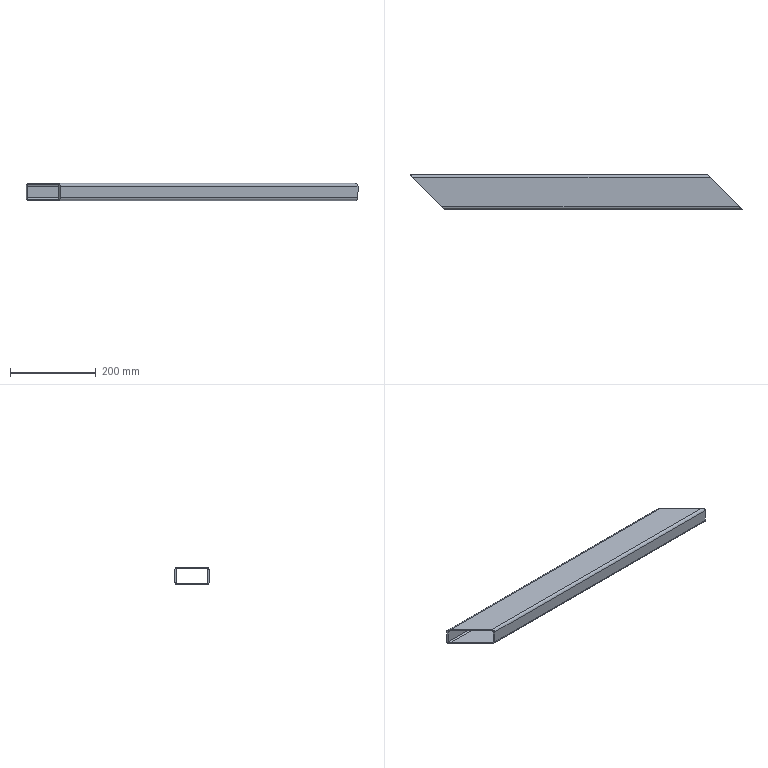Part | SolidWorks | features 3DProfileFeature 1, ICE 1, WeldMemberFeat 1, WeldmentFeature 1 | 1 solid | 18 faces | box 775 x 80 x 40 mm | volume 459272 mm3 | plane 10 | cylinder 8 | commonest cylinder face diameters 6 x4 12 x4
STEP:
#1=CARTESIAN_POINT('',(695.,40.,14.));
#2=VERTEX_POINT('',#1);
#3=CARTESIAN_POINT('',(0.,40.,14.));
#4=VERTEX_POINT('',#3);
#5=CARTESIAN_POINT('',(775.,40.,14.));
#6=DIRECTION('',(-1.,0.,0.));
#7=VECTOR('',#6,1000.);
#8=LINE('',#5,#7);
#9=EDGE_CURVE('',#2,#4,#8,.T.);
#10=ORIENTED_EDGE('',*,*,#9,.F.);
#11=CARTESIAN_POINT('',(695.,40.,-14.));
#12=VERTEX_POINT('',#11);
#13=CARTESIAN_POINT('',(695.,40.,-20.));
#14=DIRECTION('',(0.,0.,1.));
#15=VECTOR('',#14,1000.);
#16=LINE('',#13,#15);
#17=EDGE_CURVE('',#12,#2,#16,.T.);
#18=ORIENTED_EDGE('',*,*,#17,.F.);
#19=CARTESIAN_POINT('',(0.,40.,-14.));
#20=VERTEX_POINT('',#19);
#21=CARTESIAN_POINT('',(775.,40.,-14.));
#22=DIRECTION('',(-1.,0.,0.));
#23=VECTOR('',#22,1000.);
#24=LINE('',#21,#23);
#25=EDGE_CURVE('',#12,#20,#24,.T.);
#26=ORIENTED_EDGE('',*,*,#25,.T.);
#27=CARTESIAN_POINT('',(0.,40.,-14.));
#28=DIRECTION('',(0.,0.,1.));
#29=VECTOR('',#28,1000.);
#30=LINE('',#27,#29);
#31=EDGE_CURVE('',#20,#4,#30,.T.);
#32=ORIENTED_EDGE('',*,*,#31,.T.);
#33=EDGE_LOOP('',(#10,#18,#26,#32));
#34=FACE_OUTER_BOUND('',#33,.T.);
#35=CARTESIAN_POINT('',(775.,40.,-14.));
#36=DIRECTION('',(0.,-1.,0.));
#37=DIRECTION('',(0.,0.,-1.));
#38=AXIS2_PLACEMENT_3D('',#35,#36,#37);
#39=PLANE('',#38);
#40=ADVANCED_FACE('',(#34),#39,.F.);
#41=CARTESIAN_POINT('',(80.,-40.,-14.));
#42=VERTEX_POINT('',#41);
#43=CARTESIAN_POINT('',(80.,-40.,14.));
#44=VERTEX_POINT('',#43);
#45=CARTESIAN_POINT('',(80.,-40.,-20.));
#46=DIRECTION('',(0.,0.,1.));
#47=VECTOR('',#46,1000.);
#48=LINE('',#45,#47);
#49=EDGE_CURVE('',#42,#44,#48,.T.);
#50=ORIENTED_EDGE('',*,*,#49,.F.);
#51=CARTESIAN_POINT('',(775.,-40.,-14.));
#52=VERTEX_POINT('',#51);
#53=CARTESIAN_POINT('',(775.,-40.,-14.));
#54=DIRECTION('',(-1.,0.,0.));
#55=VECTOR('',#54,1000.);
#56=LINE('',#53,#55);
#57=EDGE_CURVE('',#52,#42,#56,.T.);
#58=ORIENTED_EDGE('',*,*,#57,.F.);
#59=CARTESIAN_POINT('',(775.,-40.,14.));
#60=VERTEX_POINT('',#59);
#61=CARTESIAN_POINT('',(775.,-40.,14.));
#62=DIRECTION('',(0.,0.,-1.));
#63=VECTOR('',#62,1000.);
#64=LINE('',#61,#63);
#65=EDGE_CURVE('',#60,#52,#64,.T.);
#66=ORIENTED_EDGE('',*,*,#65,.F.);
#67=CARTESIAN_POINT('',(775.,-40.,14.));
#68=DIRECTION('',(-1.,0.,0.));
#69=VECTOR('',#68,1000.);
#70=LINE('',#67,#69);
#71=EDGE_CURVE('',#60,#44,#70,.T.);
#72=ORIENTED_EDGE('',*,*,#71,.T.);
#73=EDGE_LOOP('',(#50,#58,#66,#72));
#74=FACE_OUTER_BOUND('',#73,.T.);
#75=CARTESIAN_POINT('',(775.,-40.,14.));
#76=DIRECTION('',(0.,1.,0.));
#77=DIRECTION('',(0.,0.,1.));
#78=AXIS2_PLACEMENT_3D('',#75,#76,#77);
#79=PLANE('',#78);
#80=ADVANCED_FACE('',(#74),#79,.F.);
#81=CARTESIAN_POINT('',(701.,34.,-20.));
#82=VERTEX_POINT('',#81);
#83=CARTESIAN_POINT('',(6.,34.,-20.));
#84=VERTEX_POINT('',#83);
#85=CARTESIAN_POINT('',(775.,34.,-20.));
#86=DIRECTION('',(-1.,0.,0.));
#87=VECTOR('',#86,1000.);
#88=LINE('',#85,#87);
#89=EDGE_CURVE('',#82,#84,#88,.T.);
#90=ORIENTED_EDGE('',*,*,#89,.F.);
#91=CARTESIAN_POINT('',(769.,-34.,-20.));
#92=VERTEX_POINT('',#91);
#93=CARTESIAN_POINT('',(367.5,367.5,-20.));
#94=DIRECTION('',(0.7071,-0.7071,0.));
#95=VECTOR('',#94,1000.);
#96=LINE('',#93,#95);
#97=EDGE_CURVE('',#82,#92,#96,.T.);
#98=ORIENTED_EDGE('',*,*,#97,.T.);
#99=CARTESIAN_POINT('',(74.,-34.,-20.));
#100=VERTEX_POINT('',#99);
#101=CARTESIAN_POINT('',(775.,-34.,-20.));
#102=DIRECTION('',(-1.,0.,0.));
#103=VECTOR('',#102,1000.);
#104=LINE('',#101,#103);
#105=EDGE_CURVE('',#92,#100,#104,.T.);
#106=ORIENTED_EDGE('',*,*,#105,.T.);
#107=CARTESIAN_POINT('',(20.,20.,-20.));
#108=DIRECTION('',(0.7071,-0.7071,0.));
#109=VECTOR('',#108,1000.);
#110=LINE('',#107,#109);
#111=EDGE_CURVE('',#84,#100,#110,.T.);
#112=ORIENTED_EDGE('',*,*,#111,.F.);
#113=EDGE_LOOP('',(#90,#98,#106,#112));
#114=FACE_OUTER_BOUND('',#113,.T.);
#115=CARTESIAN_POINT('',(775.,34.,-20.));
#116=DIRECTION('',(0.,0.,1.));
#117=DIRECTION('',(1.,0.,0.));
#118=AXIS2_PLACEMENT_3D('',#115,#116,#117);
#119=PLANE('',#118);
#120=ADVANCED_FACE('',(#114),#119,.F.);
#121=ORIENTED_EDGE('',*,*,#105,.F.);
#122=CARTESIAN_POINT('',(769.,-34.,-20.));
#123=CARTESIAN_POINT('',(772.515,-37.515,-20.));
#124=CARTESIAN_POINT('',(775.,-40.,-17.515));
#125=CARTESIAN_POINT('',(775.,-40.,-14.));
#126=(BOUNDED_CURVE()B_SPLINE_CURVE(3,(#122,#123,#124,#125),.UNSPECIFIED.,.F.,.F.)B_SPLINE_CURVE_WITH_KNOTS((4,4),(1.571,3.142),.UNSPECIFIED.)CURVE()GEOMETRIC_REPRESENTATION_ITEM()RATIONAL_B_SPLINE_CURVE((1.,0.8047,0.8047,1.))REPRESENTATION_ITEM(''));
#127=EDGE_CURVE('',#92,#52,#126,.T.);
#128=ORIENTED_EDGE('',*,*,#127,.T.);
#129=ORIENTED_EDGE('',*,*,#57,.T.);
#130=CARTESIAN_POINT('',(74.,-34.,-20.));
#131=CARTESIAN_POINT('',(77.515,-37.515,-20.));
#132=CARTESIAN_POINT('',(80.,-40.,-17.515));
#133=CARTESIAN_POINT('',(80.,-40.,-14.));
#134=(BOUNDED_CURVE()B_SPLINE_CURVE(3,(#130,#131,#132,#133),.UNSPECIFIED.,.F.,.F.)B_SPLINE_CURVE_WITH_KNOTS((4,4),(1.571,3.142),.UNSPECIFIED.)CURVE()GEOMETRIC_REPRESENTATION_ITEM()RATIONAL_B_SPLINE_CURVE((1.,0.8047,0.8047,1.))REPRESENTATION_ITEM(''));
#135=EDGE_CURVE('',#100,#42,#134,.T.);
#136=ORIENTED_EDGE('',*,*,#135,.F.);
#137=EDGE_LOOP('',(#121,#128,#129,#136));
#138=FACE_OUTER_BOUND('',#137,.T.);
#139=CARTESIAN_POINT('',(775.,-34.,-14.));
#140=DIRECTION('',(-1.,0.,0.));
#141=DIRECTION('',(0.,0.,1.));
#142=AXIS2_PLACEMENT_3D('',#139,#140,#141);
#143=CYLINDRICAL_SURFACE('',#142,6.);
#144=ADVANCED_FACE('',(#138),#143,.T.);
#145=ORIENTED_EDGE('',*,*,#71,.F.);
#146=CARTESIAN_POINT('',(769.,-34.,20.));
#147=VERTEX_POINT('',#146);
#148=CARTESIAN_POINT('',(775.,-40.,14.));
#149=CARTESIAN_POINT('',(775.,-40.,17.515));
#150=CARTESIAN_POINT('',(772.515,-37.515,20.));
#151=CARTESIAN_POINT('',(769.,-34.,20.));
#152=(BOUNDED_CURVE()B_SPLINE_CURVE(3,(#148,#149,#150,#151),.UNSPECIFIED.,.F.,.F.)B_SPLINE_CURVE_WITH_KNOTS((4,4),(3.142,4.712),.UNSPECIFIED.)CURVE()GEOMETRIC_REPRESENTATION_ITEM()RATIONAL_B_SPLINE_CURVE((1.,0.8047,0.8047,1.))REPRESENTATION_ITEM(''));
#153=EDGE_CURVE('',#60,#147,#152,.T.);
#154=ORIENTED_EDGE('',*,*,#153,.T.);
#155=CARTESIAN_POINT('',(74.,-34.,20.));
#156=VERTEX_POINT('',#155);
#157=CARTESIAN_POINT('',(775.,-34.,20.));
#158=DIRECTION('',(-1.,0.,0.));
#159=VECTOR('',#158,1000.);
#160=LINE('',#157,#159);
#161=EDGE_CURVE('',#147,#156,#160,.T.);
#162=ORIENTED_EDGE('',*,*,#161,.T.);
#163=CARTESIAN_POINT('',(80.,-40.,14.));
#164=CARTESIAN_POINT('',(80.,-40.,17.515));
#165=CARTESIAN_POINT('',(77.515,-37.515,20.));
#166=CARTESIAN_POINT('',(74.,-34.,20.));
#167=(BOUNDED_CURVE()B_SPLINE_CURVE(3,(#163,#164,#165,#166),.UNSPECIFIED.,.F.,.F.)B_SPLINE_CURVE_WITH_KNOTS((4,4),(3.142,4.712),.UNSPECIFIED.)CURVE()GEOMETRIC_REPRESENTATION_ITEM()RATIONAL_B_SPLINE_CURVE((1.,0.8047,0.8047,1.))REPRESENTATION_ITEM(''));
#168=EDGE_CURVE('',#44,#156,#167,.T.);
#169=ORIENTED_EDGE('',*,*,#168,.F.);
#170=EDGE_LOOP('',(#145,#154,#162,#169));
#171=FACE_OUTER_BOUND('',#170,.T.);
#172=CARTESIAN_POINT('',(775.,-34.,14.));
#173=DIRECTION('',(-1.,0.,0.));
#174=DIRECTION('',(0.,0.,1.));
#175=AXIS2_PLACEMENT_3D('',#172,#173,#174);
#176=CYLINDRICAL_SURFACE('',#175,6.);
#177=ADVANCED_FACE('',(#171),#176,.T.);
#178=ORIENTED_EDGE('',*,*,#161,.F.);
#179=CARTESIAN_POINT('',(701.,34.,20.));
#180=VERTEX_POINT('',#179);
#181=CARTESIAN_POINT('',(367.5,367.5,20.));
#182=DIRECTION('',(0.7071,-0.7071,0.));
#183=VECTOR('',#182,1000.);
#184=LINE('',#181,#183);
#185=EDGE_CURVE('',#180,#147,#184,.T.);
#186=ORIENTED_EDGE('',*,*,#185,.F.);
#187=CARTESIAN_POINT('',(6.,34.,20.));
#188=VERTEX_POINT('',#187);
#189=CARTESIAN_POINT('',(775.,34.,20.));
#190=DIRECTION('',(-1.,0.,0.));
#191=VECTOR('',#190,1000.);
#192=LINE('',#189,#191);
#193=EDGE_CURVE('',#180,#188,#192,.T.);
#194=ORIENTED_EDGE('',*,*,#193,.T.);
#195=CARTESIAN_POINT('',(20.,20.,20.));
#196=DIRECTION('',(0.7071,-0.7071,0.));
#197=VECTOR('',#196,1000.);
#198=LINE('',#195,#197);
#199=EDGE_CURVE('',#188,#156,#198,.T.);
#200=ORIENTED_EDGE('',*,*,#199,.T.);
#201=EDGE_LOOP('',(#178,#186,#194,#200));
#202=FACE_OUTER_BOUND('',#201,.T.);
#203=CARTESIAN_POINT('',(775.,-34.,20.));
#204=DIRECTION('',(0.,0.,-1.));
#205=DIRECTION('',(-1.,0.,0.));
#206=AXIS2_PLACEMENT_3D('',#203,#204,#205);
#207=PLANE('',#206);
#208=ADVANCED_FACE('',(#202),#207,.F.);
#209=ORIENTED_EDGE('',*,*,#193,.F.);
#210=CARTESIAN_POINT('',(701.,34.,20.));
#211=CARTESIAN_POINT('',(697.485,37.515,20.));
#212=CARTESIAN_POINT('',(695.,40.,17.515));
#213=CARTESIAN_POINT('',(695.,40.,14.));
#214=(BOUNDED_CURVE()B_SPLINE_CURVE(3,(#210,#211,#212,#213),.UNSPECIFIED.,.F.,.F.)B_SPLINE_CURVE_WITH_KNOTS((4,4),(4.712,6.283),.UNSPECIFIED.)CURVE()GEOMETRIC_REPRESENTATION_ITEM()RATIONAL_B_SPLINE_CURVE((1.,0.8047,0.8047,1.))REPRESENTATION_ITEM(''));
#215=EDGE_CURVE('',#180,#2,#214,.T.);
#216=ORIENTED_EDGE('',*,*,#215,.T.);
#217=ORIENTED_EDGE('',*,*,#9,.T.);
#218=CARTESIAN_POINT('',(6.,34.,20.));
#219=CARTESIAN_POINT('',(2.485,37.515,20.));
#220=CARTESIAN_POINT('',(0.,40.,17.515));
#221=CARTESIAN_POINT('',(0.,40.,14.));
#222=(BOUNDED_CURVE()B_SPLINE_CURVE(3,(#218,#219,#220,#221),.UNSPECIFIED.,.F.,.F.)B_SPLINE_CURVE_WITH_KNOTS((4,4),(4.712,6.283),.UNSPECIFIED.)CURVE()GEOMETRIC_REPRESENTATION_ITEM()RATIONAL_B_SPLINE_CURVE((1.,0.8047,0.8047,1.))REPRESENTATION_ITEM(''));
#223=EDGE_CURVE('',#188,#4,#222,.T.);
#224=ORIENTED_EDGE('',*,*,#223,.F.);
#225=EDGE_LOOP('',(#209,#216,#217,#224));
#226=FACE_OUTER_BOUND('',#225,.T.);
#227=CARTESIAN_POINT('',(775.,34.,14.));
#228=DIRECTION('',(-1.,0.,0.));
#229=DIRECTION('',(0.,0.,1.));
#230=AXIS2_PLACEMENT_3D('',#227,#228,#229);
#231=CYLINDRICAL_SURFACE('',#230,6.);
#232=ADVANCED_FACE('',(#226),#231,.T.);
#233=ORIENTED_EDGE('',*,*,#25,.F.);
#234=CARTESIAN_POINT('',(695.,40.,-14.));
#235=CARTESIAN_POINT('',(695.,40.,-17.515));
#236=CARTESIAN_POINT('',(697.485,37.515,-20.));
#237=CARTESIAN_POINT('',(701.,34.,-20.));
#238=(BOUNDED_CURVE()B_SPLINE_CURVE(3,(#234,#235,#236,#237),.UNSPECIFIED.,.F.,.F.)B_SPLINE_CURVE_WITH_KNOTS((4,4),(0.,1.571),.UNSPECIFIED.)CURVE()GEOMETRIC_REPRESENTATION_ITEM()RATIONAL_B_SPLINE_CURVE((1.,0.8047,0.8047,1.))REPRESENTATION_ITEM(''));
#239=EDGE_CURVE('',#12,#82,#238,.T.);
#240=ORIENTED_EDGE('',*,*,#239,.T.);
#241=ORIENTED_EDGE('',*,*,#89,.T.);
#242=CARTESIAN_POINT('',(0.,40.,-14.));
#243=CARTESIAN_POINT('',(0.,40.,-17.515));
#244=CARTESIAN_POINT('',(2.485,37.515,-20.));
#245=CARTESIAN_POINT('',(6.,34.,-20.));
#246=(BOUNDED_CURVE()B_SPLINE_CURVE(3,(#242,#243,#244,#245),.UNSPECIFIED.,.F.,.F.)B_SPLINE_CURVE_WITH_KNOTS((4,4),(0.,1.571),.UNSPECIFIED.)CURVE()GEOMETRIC_REPRESENTATION_ITEM()RATIONAL_B_SPLINE_CURVE((1.,0.8047,0.8047,1.))REPRESENTATION_ITEM(''));
#247=EDGE_CURVE('',#20,#84,#246,.T.);
#248=ORIENTED_EDGE('',*,*,#247,.F.);
#249=EDGE_LOOP('',(#233,#240,#241,#248));
#250=FACE_OUTER_BOUND('',#249,.T.);
#251=CARTESIAN_POINT('',(775.,34.,-14.));
#252=DIRECTION('',(-1.,0.,0.));
#253=DIRECTION('',(0.,0.,1.));
#254=AXIS2_PLACEMENT_3D('',#251,#252,#253);
#255=CYLINDRICAL_SURFACE('',#254,6.);
#256=ADVANCED_FACE('',(#250),#255,.T.);
#257=CARTESIAN_POINT('',(74.,-34.,17.));
#258=VERTEX_POINT('',#257);
#259=CARTESIAN_POINT('',(6.,34.,17.));
#260=VERTEX_POINT('',#259);
#261=CARTESIAN_POINT('',(424.5,-384.5,17.));
#262=DIRECTION('',(-0.7071,0.7071,0.));
#263=VECTOR('',#262,1000.);
#264=LINE('',#261,#263);
#265=EDGE_CURVE('',#258,#260,#264,.T.);
#266=ORIENTED_EDGE('',*,*,#265,.F.);
#267=CARTESIAN_POINT('',(77.,-37.,14.));
#268=VERTEX_POINT('',#267);
#269=CARTESIAN_POINT('',(77.,-37.,14.));
#270=CARTESIAN_POINT('',(77.,-37.,15.757));
#271=CARTESIAN_POINT('',(75.757,-35.757,17.));
#272=CARTESIAN_POINT('',(74.,-34.,17.));
#273=(BOUNDED_CURVE()B_SPLINE_CURVE(3,(#269,#270,#271,#272),.UNSPECIFIED.,.F.,.F.)B_SPLINE_CURVE_WITH_KNOTS((4,4),(3.142,4.712),.UNSPECIFIED.)CURVE()GEOMETRIC_REPRESENTATION_ITEM()RATIONAL_B_SPLINE_CURVE((1.,0.8047,0.8047,1.))REPRESENTATION_ITEM(''));
#274=EDGE_CURVE('',#268,#258,#273,.T.);
#275=ORIENTED_EDGE('',*,*,#274,.F.);
#276=CARTESIAN_POINT('',(77.,-37.,-14.));
#277=VERTEX_POINT('',#276);
#278=CARTESIAN_POINT('',(77.,-37.,14.));
#279=DIRECTION('',(0.,0.,1.));
#280=VECTOR('',#279,1000.);
#281=LINE('',#278,#280);
#282=EDGE_CURVE('',#277,#268,#281,.T.);
#283=ORIENTED_EDGE('',*,*,#282,.F.);
#284=CARTESIAN_POINT('',(74.,-34.,-17.));
#285=VERTEX_POINT('',#284);
#286=CARTESIAN_POINT('',(74.,-34.,-17.));
#287=CARTESIAN_POINT('',(75.757,-35.757,-17.));
#288=CARTESIAN_POINT('',(77.,-37.,-15.757));
#289=CARTESIAN_POINT('',(77.,-37.,-14.));
#290=(BOUNDED_CURVE()B_SPLINE_CURVE(3,(#286,#287,#288,#289),.UNSPECIFIED.,.F.,.F.)B_SPLINE_CURVE_WITH_KNOTS((4,4),(1.571,3.142),.UNSPECIFIED.)CURVE()GEOMETRIC_REPRESENTATION_ITEM()RATIONAL_B_SPLINE_CURVE((1.,0.8047,0.8047,1.))REPRESENTATION_ITEM(''));
#291=EDGE_CURVE('',#285,#277,#290,.T.);
#292=ORIENTED_EDGE('',*,*,#291,.F.);
#293=CARTESIAN_POINT('',(6.,34.,-17.));
#294=VERTEX_POINT('',#293);
#295=CARTESIAN_POINT('',(390.5,-350.5,-17.));
#296=DIRECTION('',(0.7071,-0.7071,0.));
#297=VECTOR('',#296,1000.);
#298=LINE('',#295,#297);
#299=EDGE_CURVE('',#294,#285,#298,.T.);
#300=ORIENTED_EDGE('',*,*,#299,.F.);
#301=CARTESIAN_POINT('',(3.,37.,-14.));
#302=VERTEX_POINT('',#301);
#303=CARTESIAN_POINT('',(3.,37.,-14.));
#304=CARTESIAN_POINT('',(3.,37.,-15.757));
#305=CARTESIAN_POINT('',(4.243,35.757,-17.));
#306=CARTESIAN_POINT('',(6.,34.,-17.));
#307=(BOUNDED_CURVE()B_SPLINE_CURVE(3,(#303,#304,#305,#306),.UNSPECIFIED.,.F.,.F.)B_SPLINE_CURVE_WITH_KNOTS((4,4),(0.,1.571),.UNSPECIFIED.)CURVE()GEOMETRIC_REPRESENTATION_ITEM()RATIONAL_B_SPLINE_CURVE((1.,0.8047,0.8047,1.))REPRESENTATION_ITEM(''));
#308=EDGE_CURVE('',#302,#294,#307,.T.);
#309=ORIENTED_EDGE('',*,*,#308,.F.);
#310=CARTESIAN_POINT('',(3.,37.,14.));
#311=VERTEX_POINT('',#310);
#312=CARTESIAN_POINT('',(3.,37.,-14.));
#313=DIRECTION('',(0.,0.,-1.));
#314=VECTOR('',#313,1000.);
#315=LINE('',#312,#314);
#316=EDGE_CURVE('',#311,#302,#315,.T.);
#317=ORIENTED_EDGE('',*,*,#316,.F.);
#318=CARTESIAN_POINT('',(6.,34.,17.));
#319=CARTESIAN_POINT('',(4.243,35.757,17.));
#320=CARTESIAN_POINT('',(3.,37.,15.757));
#321=CARTESIAN_POINT('',(3.,37.,14.));
#322=(BOUNDED_CURVE()B_SPLINE_CURVE(3,(#318,#319,#320,#321),.UNSPECIFIED.,.F.,.F.)B_SPLINE_CURVE_WITH_KNOTS((4,4),(4.712,6.283),.UNSPECIFIED.)CURVE()GEOMETRIC_REPRESENTATION_ITEM()RATIONAL_B_SPLINE_CURVE((1.,0.8047,0.8047,1.))REPRESENTATION_ITEM(''));
#323=EDGE_CURVE('',#260,#311,#322,.T.);
#324=ORIENTED_EDGE('',*,*,#323,.F.);
#325=EDGE_LOOP('',(#266,#275,#283,#292,#300,#309,#317,#324));
#326=FACE_BOUND('',#325,.T.);
#327=ORIENTED_EDGE('',*,*,#247,.T.);
#328=ORIENTED_EDGE('',*,*,#111,.T.);
#329=ORIENTED_EDGE('',*,*,#135,.T.);
#330=ORIENTED_EDGE('',*,*,#49,.T.);
#331=ORIENTED_EDGE('',*,*,#168,.T.);
#332=ORIENTED_EDGE('',*,*,#199,.F.);
#333=ORIENTED_EDGE('',*,*,#223,.T.);
#334=ORIENTED_EDGE('',*,*,#31,.F.);
#335=EDGE_LOOP('',(#327,#328,#329,#330,#331,#332,#333,#334));
#336=FACE_OUTER_BOUND('',#335,.T.);
#337=CARTESIAN_POINT('',(20.,20.,-20.));
#338=DIRECTION('',(-0.7071,-0.7071,0.));
#339=DIRECTION('',(0.7071,-0.7071,0.));
#340=AXIS2_PLACEMENT_3D('',#337,#338,#339);
#341=PLANE('',#340);
#342=ADVANCED_FACE('',(#326,#336),#341,.T.);
#343=CARTESIAN_POINT('',(701.,34.,17.));
#344=VERTEX_POINT('',#343);
#345=CARTESIAN_POINT('',(698.,37.,14.));
#346=VERTEX_POINT('',#345);
#347=CARTESIAN_POINT('',(701.,34.,17.));
#348=CARTESIAN_POINT('',(699.243,35.757,17.));
#349=CARTESIAN_POINT('',(698.,37.,15.757));
#350=CARTESIAN_POINT('',(698.,37.,14.));
#351=(BOUNDED_CURVE()B_SPLINE_CURVE(3,(#347,#348,#349,#350),.UNSPECIFIED.,.F.,.F.)B_SPLINE_CURVE_WITH_KNOTS((4,4),(4.712,6.283),.UNSPECIFIED.)CURVE()GEOMETRIC_REPRESENTATION_ITEM()RATIONAL_B_SPLINE_CURVE((1.,0.8047,0.8047,1.))REPRESENTATION_ITEM(''));
#352=EDGE_CURVE('',#344,#346,#351,.T.);
#353=ORIENTED_EDGE('',*,*,#352,.T.);
#354=CARTESIAN_POINT('',(698.,37.,-14.));
#355=VERTEX_POINT('',#354);
#356=CARTESIAN_POINT('',(698.,37.,-14.));
#357=DIRECTION('',(0.,0.,-1.));
#358=VECTOR('',#357,1000.);
#359=LINE('',#356,#358);
#360=EDGE_CURVE('',#346,#355,#359,.T.);
#361=ORIENTED_EDGE('',*,*,#360,.T.);
#362=CARTESIAN_POINT('',(701.,34.,-17.));
#363=VERTEX_POINT('',#362);
#364=CARTESIAN_POINT('',(698.,37.,-14.));
#365=CARTESIAN_POINT('',(698.,37.,-15.757));
#366=CARTESIAN_POINT('',(699.243,35.757,-17.));
#367=CARTESIAN_POINT('',(701.,34.,-17.));
#368=(BOUNDED_CURVE()B_SPLINE_CURVE(3,(#364,#365,#366,#367),.UNSPECIFIED.,.F.,.F.)B_SPLINE_CURVE_WITH_KNOTS((4,4),(0.,1.571),.UNSPECIFIED.)CURVE()GEOMETRIC_REPRESENTATION_ITEM()RATIONAL_B_SPLINE_CURVE((1.,0.8047,0.8047,1.))REPRESENTATION_ITEM(''));
#369=EDGE_CURVE('',#355,#363,#368,.T.);
#370=ORIENTED_EDGE('',*,*,#369,.T.);
#371=CARTESIAN_POINT('',(769.,-34.,-17.));
#372=VERTEX_POINT('',#371);
#373=CARTESIAN_POINT('',(738.,-3.,-17.));
#374=DIRECTION('',(0.7071,-0.7071,0.));
#375=VECTOR('',#374,1000.);
#376=LINE('',#373,#375);
#377=EDGE_CURVE('',#363,#372,#376,.T.);
#378=ORIENTED_EDGE('',*,*,#377,.T.);
#379=CARTESIAN_POINT('',(772.,-37.,-14.));
#380=VERTEX_POINT('',#379);
#381=CARTESIAN_POINT('',(769.,-34.,-17.));
#382=CARTESIAN_POINT('',(770.757,-35.757,-17.));
#383=CARTESIAN_POINT('',(772.,-37.,-15.757));
#384=CARTESIAN_POINT('',(772.,-37.,-14.));
#385=(BOUNDED_CURVE()B_SPLINE_CURVE(3,(#381,#382,#383,#384),.UNSPECIFIED.,.F.,.F.)B_SPLINE_CURVE_WITH_KNOTS((4,4),(1.571,3.142),.UNSPECIFIED.)CURVE()GEOMETRIC_REPRESENTATION_ITEM()RATIONAL_B_SPLINE_CURVE((1.,0.8047,0.8047,1.))REPRESENTATION_ITEM(''));
#386=EDGE_CURVE('',#372,#380,#385,.T.);
#387=ORIENTED_EDGE('',*,*,#386,.T.);
#388=CARTESIAN_POINT('',(772.,-37.,14.));
#389=VERTEX_POINT('',#388);
#390=CARTESIAN_POINT('',(772.,-37.,14.));
#391=DIRECTION('',(0.,0.,1.));
#392=VECTOR('',#391,1000.);
#393=LINE('',#390,#392);
#394=EDGE_CURVE('',#380,#389,#393,.T.);
#395=ORIENTED_EDGE('',*,*,#394,.T.);
#396=CARTESIAN_POINT('',(769.,-34.,17.));
#397=VERTEX_POINT('',#396);
#398=CARTESIAN_POINT('',(772.,-37.,14.));
#399=CARTESIAN_POINT('',(772.,-37.,15.757));
#400=CARTESIAN_POINT('',(770.757,-35.757,17.));
#401=CARTESIAN_POINT('',(769.,-34.,17.));
#402=(BOUNDED_CURVE()B_SPLINE_CURVE(3,(#398,#399,#400,#401),.UNSPECIFIED.,.F.,.F.)B_SPLINE_CURVE_WITH_KNOTS((4,4),(3.142,4.712),.UNSPECIFIED.)CURVE()GEOMETRIC_REPRESENTATION_ITEM()RATIONAL_B_SPLINE_CURVE((1.,0.8047,0.8047,1.))REPRESENTATION_ITEM(''));
#403=EDGE_CURVE('',#389,#397,#402,.T.);
#404=ORIENTED_EDGE('',*,*,#403,.T.);
#405=CARTESIAN_POINT('',(772.,-37.,17.));
#406=DIRECTION('',(-0.7071,0.7071,0.));
#407=VECTOR('',#406,1000.);
#408=LINE('',#405,#407);
#409=EDGE_CURVE('',#397,#344,#408,.T.);
#410=ORIENTED_EDGE('',*,*,#409,.T.);
#411=EDGE_LOOP('',(#353,#361,#370,#378,#387,#395,#404,#410));
#412=FACE_BOUND('',#411,.T.);
#413=ORIENTED_EDGE('',*,*,#17,.T.);
#414=ORIENTED_EDGE('',*,*,#215,.F.);
#415=ORIENTED_EDGE('',*,*,#185,.T.);
#416=ORIENTED_EDGE('',*,*,#153,.F.);
#417=ORIENTED_EDGE('',*,*,#65,.T.);
#418=ORIENTED_EDGE('',*,*,#127,.F.);
#419=ORIENTED_EDGE('',*,*,#97,.F.);
#420=ORIENTED_EDGE('',*,*,#239,.F.);
#421=EDGE_LOOP('',(#413,#414,#415,#416,#417,#418,#419,#420));
#422=FACE_OUTER_BOUND('',#421,.T.);
#423=CARTESIAN_POINT('',(367.5,367.5,-20.));
#424=DIRECTION('',(-0.7071,-0.7071,0.));
#425=DIRECTION('',(0.7071,-0.7071,0.));
#426=AXIS2_PLACEMENT_3D('',#423,#424,#425);
#427=PLANE('',#426);
#428=ADVANCED_FACE('',(#412,#422),#427,.F.);
#429=ORIENTED_EDGE('',*,*,#352,.F.);
#430=CARTESIAN_POINT('',(775.,34.,17.));
#431=DIRECTION('',(-1.,0.,0.));
#432=VECTOR('',#431,1000.);
#433=LINE('',#430,#432);
#434=EDGE_CURVE('',#344,#260,#433,.T.);
#435=ORIENTED_EDGE('',*,*,#434,.T.);
#436=ORIENTED_EDGE('',*,*,#323,.T.);
#437=CARTESIAN_POINT('',(775.,37.,14.));
#438=DIRECTION('',(-1.,0.,0.));
#439=VECTOR('',#438,1000.);
#440=LINE('',#437,#439);
#441=EDGE_CURVE('',#346,#311,#440,.T.);
#442=ORIENTED_EDGE('',*,*,#441,.F.);
#443=EDGE_LOOP('',(#429,#435,#436,#442));
#444=FACE_OUTER_BOUND('',#443,.T.);
#445=CARTESIAN_POINT('',(775.,34.,14.));
#446=DIRECTION('',(-1.,0.,0.));
#447=DIRECTION('',(0.,0.,1.));
#448=AXIS2_PLACEMENT_3D('',#445,#446,#447);
#449=CYLINDRICAL_SURFACE('',#448,3.);
#450=ADVANCED_FACE('',(#444),#449,.F.);
#451=ORIENTED_EDGE('',*,*,#360,.F.);
#452=ORIENTED_EDGE('',*,*,#441,.T.);
#453=ORIENTED_EDGE('',*,*,#316,.T.);
#454=CARTESIAN_POINT('',(775.,37.,-14.));
#455=DIRECTION('',(-1.,0.,0.));
#456=VECTOR('',#455,1000.);
#457=LINE('',#454,#456);
#458=EDGE_CURVE('',#355,#302,#457,.T.);
#459=ORIENTED_EDGE('',*,*,#458,.F.);
#460=EDGE_LOOP('',(#451,#452,#453,#459));
#461=FACE_OUTER_BOUND('',#460,.T.);
#462=CARTESIAN_POINT('',(775.,37.,-14.));
#463=DIRECTION('',(0.,-1.,0.));
#464=DIRECTION('',(0.,0.,-1.));
#465=AXIS2_PLACEMENT_3D('',#462,#463,#464);
#466=PLANE('',#465);
#467=ADVANCED_FACE('',(#461),#466,.T.);
#468=ORIENTED_EDGE('',*,*,#369,.F.);
#469=ORIENTED_EDGE('',*,*,#458,.T.);
#470=ORIENTED_EDGE('',*,*,#308,.T.);
#471=CARTESIAN_POINT('',(775.,34.,-17.));
#472=DIRECTION('',(-1.,0.,0.));
#473=VECTOR('',#472,1000.);
#474=LINE('',#471,#473);
#475=EDGE_CURVE('',#363,#294,#474,.T.);
#476=ORIENTED_EDGE('',*,*,#475,.F.);
#477=EDGE_LOOP('',(#468,#469,#470,#476));
#478=FACE_OUTER_BOUND('',#477,.T.);
#479=CARTESIAN_POINT('',(775.,34.,-14.));
#480=DIRECTION('',(-1.,0.,0.));
#481=DIRECTION('',(0.,0.,1.));
#482=AXIS2_PLACEMENT_3D('',#479,#480,#481);
#483=CYLINDRICAL_SURFACE('',#482,3.);
#484=ADVANCED_FACE('',(#478),#483,.F.);
#485=ORIENTED_EDGE('',*,*,#377,.F.);
#486=ORIENTED_EDGE('',*,*,#475,.T.);
#487=ORIENTED_EDGE('',*,*,#299,.T.);
#488=CARTESIAN_POINT('',(775.,-34.,-17.));
#489=DIRECTION('',(-1.,0.,0.));
#490=VECTOR('',#489,1000.);
#491=LINE('',#488,#490);
#492=EDGE_CURVE('',#372,#285,#491,.T.);
#493=ORIENTED_EDGE('',*,*,#492,.F.);
#494=EDGE_LOOP('',(#485,#486,#487,#493));
#495=FACE_OUTER_BOUND('',#494,.T.);
#496=CARTESIAN_POINT('',(775.,34.,-17.));
#497=DIRECTION('',(0.,0.,1.));
#498=DIRECTION('',(1.,0.,0.));
#499=AXIS2_PLACEMENT_3D('',#496,#497,#498);
#500=PLANE('',#499);
#501=ADVANCED_FACE('',(#495),#500,.T.);
#502=ORIENTED_EDGE('',*,*,#386,.F.);
#503=ORIENTED_EDGE('',*,*,#492,.T.);
#504=ORIENTED_EDGE('',*,*,#291,.T.);
#505=CARTESIAN_POINT('',(775.,-37.,-14.));
#506=DIRECTION('',(-1.,0.,0.));
#507=VECTOR('',#506,1000.);
#508=LINE('',#505,#507);
#509=EDGE_CURVE('',#380,#277,#508,.T.);
#510=ORIENTED_EDGE('',*,*,#509,.F.);
#511=EDGE_LOOP('',(#502,#503,#504,#510));
#512=FACE_OUTER_BOUND('',#511,.T.);
#513=CARTESIAN_POINT('',(775.,-34.,-14.));
#514=DIRECTION('',(-1.,0.,0.));
#515=DIRECTION('',(0.,0.,1.));
#516=AXIS2_PLACEMENT_3D('',#513,#514,#515);
#517=CYLINDRICAL_SURFACE('',#516,3.);
#518=ADVANCED_FACE('',(#512),#517,.F.);
#519=ORIENTED_EDGE('',*,*,#394,.F.);
#520=ORIENTED_EDGE('',*,*,#509,.T.);
#521=ORIENTED_EDGE('',*,*,#282,.T.);
#522=CARTESIAN_POINT('',(775.,-37.,14.));
#523=DIRECTION('',(-1.,0.,0.));
#524=VECTOR('',#523,1000.);
#525=LINE('',#522,#524);
#526=EDGE_CURVE('',#389,#268,#525,.T.);
#527=ORIENTED_EDGE('',*,*,#526,.F.);
#528=EDGE_LOOP('',(#519,#520,#521,#527));
#529=FACE_OUTER_BOUND('',#528,.T.);
#530=CARTESIAN_POINT('',(775.,-37.,14.));
#531=DIRECTION('',(0.,1.,0.));
#532=DIRECTION('',(0.,0.,1.));
#533=AXIS2_PLACEMENT_3D('',#530,#531,#532);
#534=PLANE('',#533);
#535=ADVANCED_FACE('',(#529),#534,.T.);
#536=ORIENTED_EDGE('',*,*,#403,.F.);
#537=ORIENTED_EDGE('',*,*,#526,.T.);
#538=ORIENTED_EDGE('',*,*,#274,.T.);
#539=CARTESIAN_POINT('',(775.,-34.,17.));
#540=DIRECTION('',(-1.,0.,0.));
#541=VECTOR('',#540,1000.);
#542=LINE('',#539,#541);
#543=EDGE_CURVE('',#397,#258,#542,.T.);
#544=ORIENTED_EDGE('',*,*,#543,.F.);
#545=EDGE_LOOP('',(#536,#537,#538,#544));
#546=FACE_OUTER_BOUND('',#545,.T.);
#547=CARTESIAN_POINT('',(775.,-34.,14.));
#548=DIRECTION('',(-1.,0.,0.));
#549=DIRECTION('',(0.,0.,1.));
#550=AXIS2_PLACEMENT_3D('',#547,#548,#549);
#551=CYLINDRICAL_SURFACE('',#550,3.);
#552=ADVANCED_FACE('',(#546),#551,.F.);
#553=ORIENTED_EDGE('',*,*,#409,.F.);
#554=ORIENTED_EDGE('',*,*,#543,.T.);
#555=ORIENTED_EDGE('',*,*,#265,.T.);
#556=ORIENTED_EDGE('',*,*,#434,.F.);
#557=EDGE_LOOP('',(#553,#554,#555,#556));
#558=FACE_OUTER_BOUND('',#557,.T.);
#559=CARTESIAN_POINT('',(775.,-34.,17.));
#560=DIRECTION('',(0.,0.,-1.));
#561=DIRECTION('',(-1.,0.,0.));
#562=AXIS2_PLACEMENT_3D('',#559,#560,#561);
#563=PLANE('',#562);
#564=ADVANCED_FACE('',(#558),#563,.T.);
#565=CLOSED_SHELL('',(#40,#80,#120,#144,#177,#208,#232,#256,#342,#428,#450,#467,#484,#501,#518,#535,#552,#564));
#566=MANIFOLD_SOLID_BREP('',#565);
#567=CARTESIAN_POINT('',(0.,0.,0.));
#568=DIRECTION('',(0.,0.,1.));
#569=DIRECTION('',(1.,0.,0.));
#570=AXIS2_PLACEMENT_3D('',#567,#568,#569);
#571=(LENGTH_UNIT()NAMED_UNIT(*)SI_UNIT(.MILLI.,.METRE.));
#572=UNCERTAINTY_MEASURE_WITH_UNIT(LENGTH_MEASURE(0.00001),#571,'','');
#573=(NAMED_UNIT(*)PLANE_ANGLE_UNIT()SI_UNIT($,.RADIAN.));
#574=(NAMED_UNIT(*)SI_UNIT($,.STERADIAN.)SOLID_ANGLE_UNIT());
#575=(GEOMETRIC_REPRESENTATION_CONTEXT(3)GLOBAL_UNCERTAINTY_ASSIGNED_CONTEXT((#572))GLOBAL_UNIT_ASSIGNED_CONTEXT((#571,#573,#574))REPRESENTATION_CONTEXT('',''));
#576=ADVANCED_BREP_SHAPE_REPRESENTATION('',(#566,#570),#575);